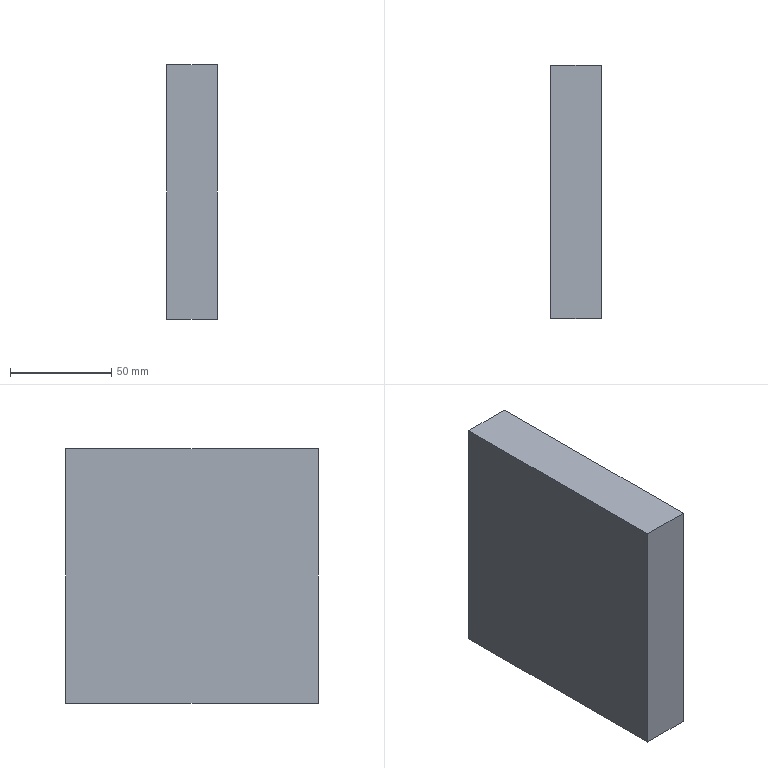Part | SolidWorks | features Extrusion 1 | 1 solid | 6 faces | box 25 x 125 x 126 mm | volume 393750 mm3 | plane 6
STEP:
#1=CARTESIAN_POINT('',(-12.5,-62.5,-63.));
#2=VERTEX_POINT('',#1);
#3=CARTESIAN_POINT('',(-12.5,-62.5,63.));
#4=VERTEX_POINT('',#3);
#5=CARTESIAN_POINT('',(-12.5,-62.5,-63.));
#6=DIRECTION('',(0.,0.,1.));
#7=VECTOR('',#6,1000.);
#8=LINE('',#5,#7);
#9=EDGE_CURVE('',#2,#4,#8,.T.);
#10=ORIENTED_EDGE('',*,*,#9,.T.);
#11=CARTESIAN_POINT('',(-12.5,62.5,63.));
#12=VERTEX_POINT('',#11);
#13=CARTESIAN_POINT('',(-12.5,62.5,63.));
#14=DIRECTION('',(0.,-1.,0.));
#15=VECTOR('',#14,1000.);
#16=LINE('',#13,#15);
#17=EDGE_CURVE('',#12,#4,#16,.T.);
#18=ORIENTED_EDGE('',*,*,#17,.F.);
#19=CARTESIAN_POINT('',(-12.5,62.5,-63.));
#20=VERTEX_POINT('',#19);
#21=CARTESIAN_POINT('',(-12.5,62.5,-63.));
#22=DIRECTION('',(0.,0.,1.));
#23=VECTOR('',#22,1000.);
#24=LINE('',#21,#23);
#25=EDGE_CURVE('',#20,#12,#24,.T.);
#26=ORIENTED_EDGE('',*,*,#25,.F.);
#27=CARTESIAN_POINT('',(-12.5,62.5,-63.));
#28=DIRECTION('',(0.,-1.,0.));
#29=VECTOR('',#28,1000.);
#30=LINE('',#27,#29);
#31=EDGE_CURVE('',#20,#2,#30,.T.);
#32=ORIENTED_EDGE('',*,*,#31,.T.);
#33=EDGE_LOOP('',(#10,#18,#26,#32));
#34=FACE_OUTER_BOUND('',#33,.T.);
#35=CARTESIAN_POINT('',(-12.5,62.5,-63.));
#36=DIRECTION('',(1.,0.,0.));
#37=DIRECTION('',(0.,0.,-1.));
#38=AXIS2_PLACEMENT_3D('',#35,#36,#37);
#39=PLANE('',#38);
#40=ADVANCED_FACE('',(#34),#39,.F.);
#41=CARTESIAN_POINT('',(12.5,-62.5,63.));
#42=VERTEX_POINT('',#41);
#43=CARTESIAN_POINT('',(-12.5,-62.5,63.));
#44=DIRECTION('',(1.,0.,0.));
#45=VECTOR('',#44,1000.);
#46=LINE('',#43,#45);
#47=EDGE_CURVE('',#4,#42,#46,.T.);
#48=ORIENTED_EDGE('',*,*,#47,.T.);
#49=CARTESIAN_POINT('',(12.5,62.5,63.));
#50=VERTEX_POINT('',#49);
#51=CARTESIAN_POINT('',(12.5,62.5,63.));
#52=DIRECTION('',(0.,-1.,0.));
#53=VECTOR('',#52,1000.);
#54=LINE('',#51,#53);
#55=EDGE_CURVE('',#50,#42,#54,.T.);
#56=ORIENTED_EDGE('',*,*,#55,.F.);
#57=CARTESIAN_POINT('',(-12.5,62.5,63.));
#58=DIRECTION('',(1.,0.,0.));
#59=VECTOR('',#58,1000.);
#60=LINE('',#57,#59);
#61=EDGE_CURVE('',#12,#50,#60,.T.);
#62=ORIENTED_EDGE('',*,*,#61,.F.);
#63=ORIENTED_EDGE('',*,*,#17,.T.);
#64=EDGE_LOOP('',(#48,#56,#62,#63));
#65=FACE_OUTER_BOUND('',#64,.T.);
#66=CARTESIAN_POINT('',(-12.5,62.5,63.));
#67=DIRECTION('',(0.,0.,-1.));
#68=DIRECTION('',(-1.,0.,0.));
#69=AXIS2_PLACEMENT_3D('',#66,#67,#68);
#70=PLANE('',#69);
#71=ADVANCED_FACE('',(#65),#70,.F.);
#72=CARTESIAN_POINT('',(12.5,-62.5,-63.));
#73=VERTEX_POINT('',#72);
#74=CARTESIAN_POINT('',(12.5,-62.5,-63.));
#75=DIRECTION('',(0.,0.,-1.));
#76=VECTOR('',#75,1000.);
#77=LINE('',#74,#76);
#78=EDGE_CURVE('',#42,#73,#77,.T.);
#79=ORIENTED_EDGE('',*,*,#78,.T.);
#80=CARTESIAN_POINT('',(12.5,62.5,-63.));
#81=VERTEX_POINT('',#80);
#82=CARTESIAN_POINT('',(12.5,62.5,-63.));
#83=DIRECTION('',(0.,-1.,0.));
#84=VECTOR('',#83,1000.);
#85=LINE('',#82,#84);
#86=EDGE_CURVE('',#81,#73,#85,.T.);
#87=ORIENTED_EDGE('',*,*,#86,.F.);
#88=CARTESIAN_POINT('',(12.5,62.5,-63.));
#89=DIRECTION('',(0.,0.,-1.));
#90=VECTOR('',#89,1000.);
#91=LINE('',#88,#90);
#92=EDGE_CURVE('',#50,#81,#91,.T.);
#93=ORIENTED_EDGE('',*,*,#92,.F.);
#94=ORIENTED_EDGE('',*,*,#55,.T.);
#95=EDGE_LOOP('',(#79,#87,#93,#94));
#96=FACE_OUTER_BOUND('',#95,.T.);
#97=CARTESIAN_POINT('',(12.5,62.5,-63.));
#98=DIRECTION('',(-1.,0.,0.));
#99=DIRECTION('',(0.,0.,1.));
#100=AXIS2_PLACEMENT_3D('',#97,#98,#99);
#101=PLANE('',#100);
#102=ADVANCED_FACE('',(#96),#101,.F.);
#103=CARTESIAN_POINT('',(-12.5,-62.5,-63.));
#104=DIRECTION('',(-1.,0.,0.));
#105=VECTOR('',#104,1000.);
#106=LINE('',#103,#105);
#107=EDGE_CURVE('',#73,#2,#106,.T.);
#108=ORIENTED_EDGE('',*,*,#107,.T.);
#109=ORIENTED_EDGE('',*,*,#31,.F.);
#110=CARTESIAN_POINT('',(-12.5,62.5,-63.));
#111=DIRECTION('',(-1.,0.,0.));
#112=VECTOR('',#111,1000.);
#113=LINE('',#110,#112);
#114=EDGE_CURVE('',#81,#20,#113,.T.);
#115=ORIENTED_EDGE('',*,*,#114,.F.);
#116=ORIENTED_EDGE('',*,*,#86,.T.);
#117=EDGE_LOOP('',(#108,#109,#115,#116));
#118=FACE_OUTER_BOUND('',#117,.T.);
#119=CARTESIAN_POINT('',(-12.5,62.5,-63.));
#120=DIRECTION('',(0.,0.,1.));
#121=DIRECTION('',(1.,0.,0.));
#122=AXIS2_PLACEMENT_3D('',#119,#120,#121);
#123=PLANE('',#122);
#124=ADVANCED_FACE('',(#118),#123,.F.);
#125=ORIENTED_EDGE('',*,*,#25,.T.);
#126=ORIENTED_EDGE('',*,*,#61,.T.);
#127=ORIENTED_EDGE('',*,*,#92,.T.);
#128=ORIENTED_EDGE('',*,*,#114,.T.);
#129=EDGE_LOOP('',(#125,#126,#127,#128));
#130=FACE_OUTER_BOUND('',#129,.T.);
#131=CARTESIAN_POINT('',(0.,62.5,0.));
#132=DIRECTION('',(0.,1.,0.));
#133=DIRECTION('',(0.,0.,1.));
#134=AXIS2_PLACEMENT_3D('',#131,#132,#133);
#135=PLANE('',#134);
#136=ADVANCED_FACE('',(#130),#135,.T.);
#137=ORIENTED_EDGE('',*,*,#9,.F.);
#138=ORIENTED_EDGE('',*,*,#107,.F.);
#139=ORIENTED_EDGE('',*,*,#78,.F.);
#140=ORIENTED_EDGE('',*,*,#47,.F.);
#141=EDGE_LOOP('',(#137,#138,#139,#140));
#142=FACE_OUTER_BOUND('',#141,.T.);
#143=CARTESIAN_POINT('',(0.,-62.5,0.));
#144=DIRECTION('',(0.,1.,0.));
#145=DIRECTION('',(0.,0.,1.));
#146=AXIS2_PLACEMENT_3D('',#143,#144,#145);
#147=PLANE('',#146);
#148=ADVANCED_FACE('',(#142),#147,.F.);
#149=CLOSED_SHELL('',(#40,#71,#102,#124,#136,#148));
#150=MANIFOLD_SOLID_BREP('',#149);
#151=CARTESIAN_POINT('',(0.,0.,0.));
#152=DIRECTION('',(0.,0.,1.));
#153=DIRECTION('',(1.,0.,0.));
#154=AXIS2_PLACEMENT_3D('',#151,#152,#153);
#155=(LENGTH_UNIT()NAMED_UNIT(*)SI_UNIT(.MILLI.,.METRE.));
#156=UNCERTAINTY_MEASURE_WITH_UNIT(LENGTH_MEASURE(0.00001),#155,'','');
#157=(NAMED_UNIT(*)PLANE_ANGLE_UNIT()SI_UNIT($,.RADIAN.));
#158=(NAMED_UNIT(*)SI_UNIT($,.STERADIAN.)SOLID_ANGLE_UNIT());
#159=(GEOMETRIC_REPRESENTATION_CONTEXT(3)GLOBAL_UNCERTAINTY_ASSIGNED_CONTEXT((#156))GLOBAL_UNIT_ASSIGNED_CONTEXT((#155,#157,#158))REPRESENTATION_CONTEXT('',''));
#160=ADVANCED_BREP_SHAPE_REPRESENTATION('',(#150,#154),#159);